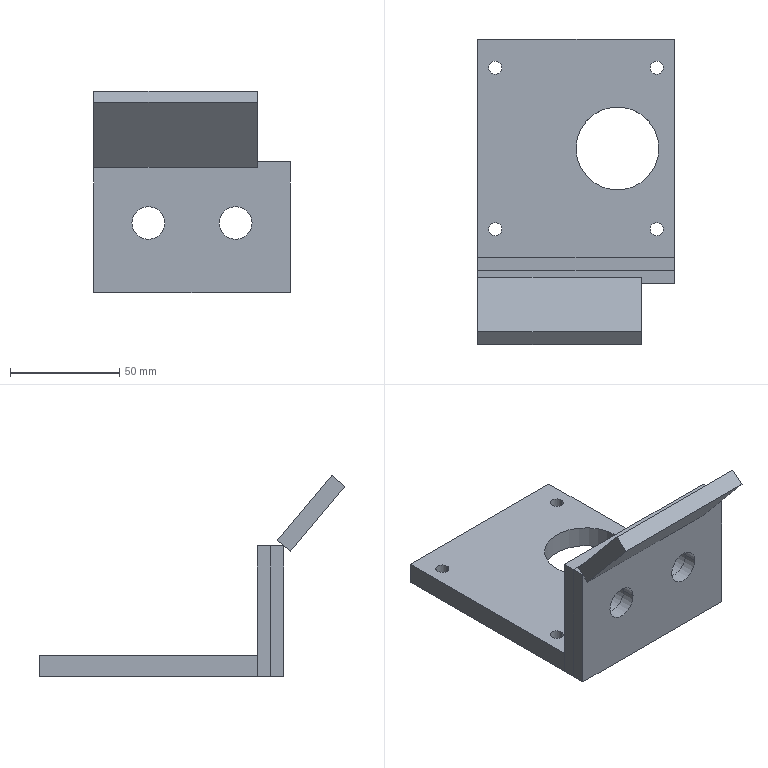Part | SolidWorks | features ICE 4, BossThin 1, Extrusion 1 | 4 solids | 42 faces | box 90 x 140.048 x 92.376 mm | volume 160839 mm3 | plane 24 | cylinder 18 | commonest cylinder face diameters 6 x8 15 x8 38 x2
STEP:
#1=CARTESIAN_POINT('',(-40.,-37.,10.));
#2=VERTEX_POINT('',#1);
#3=CARTESIAN_POINT('',(-34.,-37.,10.));
#4=VERTEX_POINT('',#3);
#5=CARTESIAN_POINT('',(-37.,-37.,10.));
#6=DIRECTION('',(0.,0.,1.));
#7=DIRECTION('',(-1.,0.,0.));
#8=AXIS2_PLACEMENT_3D('',#5,#6,#7);
#9=CIRCLE('',#8,3.);
#10=EDGE_CURVE('',#2,#4,#9,.T.);
#11=ORIENTED_EDGE('',*,*,#10,.T.);
#12=CARTESIAN_POINT('',(-34.,-37.,0.));
#13=VERTEX_POINT('',#12);
#14=CARTESIAN_POINT('',(-34.,-37.,10.));
#15=DIRECTION('',(0.,0.,-1.));
#16=VECTOR('',#15,1000.);
#17=LINE('',#14,#16);
#18=EDGE_CURVE('',#4,#13,#17,.T.);
#19=ORIENTED_EDGE('',*,*,#18,.T.);
#20=CARTESIAN_POINT('',(-40.,-37.,0.));
#21=VERTEX_POINT('',#20);
#22=CARTESIAN_POINT('',(-37.,-37.,0.));
#23=DIRECTION('',(0.,0.,1.));
#24=DIRECTION('',(-1.,0.,0.));
#25=AXIS2_PLACEMENT_3D('',#22,#23,#24);
#26=CIRCLE('',#25,3.);
#27=EDGE_CURVE('',#21,#13,#26,.T.);
#28=ORIENTED_EDGE('',*,*,#27,.F.);
#29=CARTESIAN_POINT('',(-40.,-37.,10.));
#30=DIRECTION('',(0.,0.,-1.));
#31=VECTOR('',#30,1000.);
#32=LINE('',#29,#31);
#33=EDGE_CURVE('',#2,#21,#32,.T.);
#34=ORIENTED_EDGE('',*,*,#33,.F.);
#35=EDGE_LOOP('',(#11,#19,#28,#34));
#36=FACE_OUTER_BOUND('',#35,.T.);
#37=CARTESIAN_POINT('',(-37.,-37.,10.));
#38=DIRECTION('',(0.,0.,-1.));
#39=DIRECTION('',(-1.,0.,0.));
#40=AXIS2_PLACEMENT_3D('',#37,#38,#39);
#41=CYLINDRICAL_SURFACE('',#40,3.);
#42=ADVANCED_FACE('',(#36),#41,.F.);
#43=CARTESIAN_POINT('',(34.,-37.,10.));
#44=VERTEX_POINT('',#43);
#45=CARTESIAN_POINT('',(40.,-37.,10.));
#46=VERTEX_POINT('',#45);
#47=CARTESIAN_POINT('',(37.,-37.,10.));
#48=DIRECTION('',(0.,0.,1.));
#49=DIRECTION('',(1.,0.,0.));
#50=AXIS2_PLACEMENT_3D('',#47,#48,#49);
#51=CIRCLE('',#50,3.);
#52=EDGE_CURVE('',#44,#46,#51,.T.);
#53=ORIENTED_EDGE('',*,*,#52,.T.);
#54=CARTESIAN_POINT('',(40.,-37.,0.));
#55=VERTEX_POINT('',#54);
#56=CARTESIAN_POINT('',(40.,-37.,10.));
#57=DIRECTION('',(0.,0.,-1.));
#58=VECTOR('',#57,1000.);
#59=LINE('',#56,#58);
#60=EDGE_CURVE('',#46,#55,#59,.T.);
#61=ORIENTED_EDGE('',*,*,#60,.T.);
#62=CARTESIAN_POINT('',(34.,-37.,0.));
#63=VERTEX_POINT('',#62);
#64=CARTESIAN_POINT('',(37.,-37.,0.));
#65=DIRECTION('',(0.,0.,1.));
#66=DIRECTION('',(1.,0.,0.));
#67=AXIS2_PLACEMENT_3D('',#64,#65,#66);
#68=CIRCLE('',#67,3.);
#69=EDGE_CURVE('',#63,#55,#68,.T.);
#70=ORIENTED_EDGE('',*,*,#69,.F.);
#71=CARTESIAN_POINT('',(34.,-37.,10.));
#72=DIRECTION('',(0.,0.,-1.));
#73=VECTOR('',#72,1000.);
#74=LINE('',#71,#73);
#75=EDGE_CURVE('',#44,#63,#74,.T.);
#76=ORIENTED_EDGE('',*,*,#75,.F.);
#77=EDGE_LOOP('',(#53,#61,#70,#76));
#78=FACE_OUTER_BOUND('',#77,.T.);
#79=CARTESIAN_POINT('',(37.,-37.,10.));
#80=DIRECTION('',(0.,0.,-1.));
#81=DIRECTION('',(-1.,0.,0.));
#82=AXIS2_PLACEMENT_3D('',#79,#80,#81);
#83=CYLINDRICAL_SURFACE('',#82,3.);
#84=ADVANCED_FACE('',(#78),#83,.F.);
#85=CARTESIAN_POINT('',(-40.,37.,10.));
#86=VERTEX_POINT('',#85);
#87=CARTESIAN_POINT('',(-34.,37.,10.));
#88=VERTEX_POINT('',#87);
#89=CARTESIAN_POINT('',(-37.,37.,10.));
#90=DIRECTION('',(0.,0.,1.));
#91=DIRECTION('',(1.,0.,0.));
#92=AXIS2_PLACEMENT_3D('',#89,#90,#91);
#93=CIRCLE('',#92,3.);
#94=EDGE_CURVE('',#86,#88,#93,.T.);
#95=ORIENTED_EDGE('',*,*,#94,.T.);
#96=CARTESIAN_POINT('',(-34.,37.,0.));
#97=VERTEX_POINT('',#96);
#98=CARTESIAN_POINT('',(-34.,37.,10.));
#99=DIRECTION('',(0.,0.,-1.));
#100=VECTOR('',#99,1000.);
#101=LINE('',#98,#100);
#102=EDGE_CURVE('',#88,#97,#101,.T.);
#103=ORIENTED_EDGE('',*,*,#102,.T.);
#104=CARTESIAN_POINT('',(-40.,37.,0.));
#105=VERTEX_POINT('',#104);
#106=CARTESIAN_POINT('',(-37.,37.,0.));
#107=DIRECTION('',(0.,0.,1.));
#108=DIRECTION('',(1.,0.,0.));
#109=AXIS2_PLACEMENT_3D('',#106,#107,#108);
#110=CIRCLE('',#109,3.);
#111=EDGE_CURVE('',#105,#97,#110,.T.);
#112=ORIENTED_EDGE('',*,*,#111,.F.);
#113=CARTESIAN_POINT('',(-40.,37.,10.));
#114=DIRECTION('',(0.,0.,-1.));
#115=VECTOR('',#114,1000.);
#116=LINE('',#113,#115);
#117=EDGE_CURVE('',#86,#105,#116,.T.);
#118=ORIENTED_EDGE('',*,*,#117,.F.);
#119=EDGE_LOOP('',(#95,#103,#112,#118));
#120=FACE_OUTER_BOUND('',#119,.T.);
#121=CARTESIAN_POINT('',(-37.,37.,10.));
#122=DIRECTION('',(0.,0.,-1.));
#123=DIRECTION('',(-1.,0.,0.));
#124=AXIS2_PLACEMENT_3D('',#121,#122,#123);
#125=CYLINDRICAL_SURFACE('',#124,3.);
#126=ADVANCED_FACE('',(#120),#125,.F.);
#127=CARTESIAN_POINT('',(34.,37.,10.));
#128=VERTEX_POINT('',#127);
#129=CARTESIAN_POINT('',(40.,37.,10.));
#130=VERTEX_POINT('',#129);
#131=CARTESIAN_POINT('',(37.,37.,10.));
#132=DIRECTION('',(0.,0.,1.));
#133=DIRECTION('',(-1.,0.,0.));
#134=AXIS2_PLACEMENT_3D('',#131,#132,#133);
#135=CIRCLE('',#134,3.);
#136=EDGE_CURVE('',#128,#130,#135,.T.);
#137=ORIENTED_EDGE('',*,*,#136,.T.);
#138=CARTESIAN_POINT('',(40.,37.,0.));
#139=VERTEX_POINT('',#138);
#140=CARTESIAN_POINT('',(40.,37.,10.));
#141=DIRECTION('',(0.,0.,-1.));
#142=VECTOR('',#141,1000.);
#143=LINE('',#140,#142);
#144=EDGE_CURVE('',#130,#139,#143,.T.);
#145=ORIENTED_EDGE('',*,*,#144,.T.);
#146=CARTESIAN_POINT('',(34.,37.,0.));
#147=VERTEX_POINT('',#146);
#148=CARTESIAN_POINT('',(37.,37.,0.));
#149=DIRECTION('',(0.,0.,1.));
#150=DIRECTION('',(-1.,0.,0.));
#151=AXIS2_PLACEMENT_3D('',#148,#149,#150);
#152=CIRCLE('',#151,3.);
#153=EDGE_CURVE('',#147,#139,#152,.T.);
#154=ORIENTED_EDGE('',*,*,#153,.F.);
#155=CARTESIAN_POINT('',(34.,37.,10.));
#156=DIRECTION('',(0.,0.,-1.));
#157=VECTOR('',#156,1000.);
#158=LINE('',#155,#157);
#159=EDGE_CURVE('',#128,#147,#158,.T.);
#160=ORIENTED_EDGE('',*,*,#159,.F.);
#161=EDGE_LOOP('',(#137,#145,#154,#160));
#162=FACE_OUTER_BOUND('',#161,.T.);
#163=CARTESIAN_POINT('',(37.,37.,10.));
#164=DIRECTION('',(0.,0.,-1.));
#165=DIRECTION('',(-1.,0.,0.));
#166=AXIS2_PLACEMENT_3D('',#163,#164,#165);
#167=CYLINDRICAL_SURFACE('',#166,3.);
#168=ADVANCED_FACE('',(#162),#167,.F.);
#169=CARTESIAN_POINT('',(0.,0.,10.));
#170=VERTEX_POINT('',#169);
#171=CARTESIAN_POINT('',(38.,0.,10.));
#172=VERTEX_POINT('',#171);
#173=CARTESIAN_POINT('',(19.,0.,10.));
#174=DIRECTION('',(0.,0.,1.));
#175=DIRECTION('',(1.,0.,0.));
#176=AXIS2_PLACEMENT_3D('',#173,#174,#175);
#177=CIRCLE('',#176,19.);
#178=EDGE_CURVE('',#170,#172,#177,.T.);
#179=ORIENTED_EDGE('',*,*,#178,.T.);
#180=CARTESIAN_POINT('',(38.,0.,0.));
#181=VERTEX_POINT('',#180);
#182=CARTESIAN_POINT('',(38.,0.,10.));
#183=DIRECTION('',(0.,0.,-1.));
#184=VECTOR('',#183,1000.);
#185=LINE('',#182,#184);
#186=EDGE_CURVE('',#172,#181,#185,.T.);
#187=ORIENTED_EDGE('',*,*,#186,.T.);
#188=CARTESIAN_POINT('',(0.,0.,0.));
#189=VERTEX_POINT('',#188);
#190=CARTESIAN_POINT('',(19.,0.,0.));
#191=DIRECTION('',(0.,0.,1.));
#192=DIRECTION('',(1.,0.,0.));
#193=AXIS2_PLACEMENT_3D('',#190,#191,#192);
#194=CIRCLE('',#193,19.);
#195=EDGE_CURVE('',#189,#181,#194,.T.);
#196=ORIENTED_EDGE('',*,*,#195,.F.);
#197=CARTESIAN_POINT('',(0.,0.,10.));
#198=DIRECTION('',(0.,0.,-1.));
#199=VECTOR('',#198,1000.);
#200=LINE('',#197,#199);
#201=EDGE_CURVE('',#170,#189,#200,.T.);
#202=ORIENTED_EDGE('',*,*,#201,.F.);
#203=EDGE_LOOP('',(#179,#187,#196,#202));
#204=FACE_OUTER_BOUND('',#203,.T.);
#205=CARTESIAN_POINT('',(19.,0.,10.));
#206=DIRECTION('',(0.,0.,-1.));
#207=DIRECTION('',(-1.,0.,0.));
#208=AXIS2_PLACEMENT_3D('',#205,#206,#207);
#209=CYLINDRICAL_SURFACE('',#208,19.);
#210=ADVANCED_FACE('',(#204),#209,.F.);
#211=CARTESIAN_POINT('',(45.,-50.,10.));
#212=VERTEX_POINT('',#211);
#213=CARTESIAN_POINT('',(45.,50.,10.));
#214=VERTEX_POINT('',#213);
#215=CARTESIAN_POINT('',(45.,-50.,10.));
#216=DIRECTION('',(0.,1.,0.));
#217=VECTOR('',#216,1000.);
#218=LINE('',#215,#217);
#219=EDGE_CURVE('',#212,#214,#218,.T.);
#220=ORIENTED_EDGE('',*,*,#219,.T.);
#221=CARTESIAN_POINT('',(-45.,50.,10.));
#222=VERTEX_POINT('',#221);
#223=CARTESIAN_POINT('',(-45.,50.,10.));
#224=DIRECTION('',(-1.,0.,0.));
#225=VECTOR('',#224,1000.);
#226=LINE('',#223,#225);
#227=EDGE_CURVE('',#214,#222,#226,.T.);
#228=ORIENTED_EDGE('',*,*,#227,.T.);
#229=CARTESIAN_POINT('',(-45.,-50.,10.));
#230=VERTEX_POINT('',#229);
#231=CARTESIAN_POINT('',(-45.,-50.,10.));
#232=DIRECTION('',(0.,-1.,0.));
#233=VECTOR('',#232,1000.);
#234=LINE('',#231,#233);
#235=EDGE_CURVE('',#222,#230,#234,.T.);
#236=ORIENTED_EDGE('',*,*,#235,.T.);
#237=CARTESIAN_POINT('',(-45.,-50.,10.));
#238=DIRECTION('',(1.,0.,0.));
#239=VECTOR('',#238,1000.);
#240=LINE('',#237,#239);
#241=EDGE_CURVE('',#230,#212,#240,.T.);
#242=ORIENTED_EDGE('',*,*,#241,.T.);
#243=EDGE_LOOP('',(#220,#228,#236,#242));
#244=FACE_OUTER_BOUND('',#243,.T.);
#245=ORIENTED_EDGE('',*,*,#178,.F.);
#246=CARTESIAN_POINT('',(19.,0.,10.));
#247=DIRECTION('',(0.,0.,1.));
#248=DIRECTION('',(1.,0.,0.));
#249=AXIS2_PLACEMENT_3D('',#246,#247,#248);
#250=CIRCLE('',#249,19.);
#251=EDGE_CURVE('',#172,#170,#250,.T.);
#252=ORIENTED_EDGE('',*,*,#251,.F.);
#253=EDGE_LOOP('',(#245,#252));
#254=FACE_BOUND('',#253,.T.);
#255=ORIENTED_EDGE('',*,*,#136,.F.);
#256=CARTESIAN_POINT('',(37.,37.,10.));
#257=DIRECTION('',(0.,0.,1.));
#258=DIRECTION('',(-1.,0.,0.));
#259=AXIS2_PLACEMENT_3D('',#256,#257,#258);
#260=CIRCLE('',#259,3.);
#261=EDGE_CURVE('',#130,#128,#260,.T.);
#262=ORIENTED_EDGE('',*,*,#261,.F.);
#263=EDGE_LOOP('',(#255,#262));
#264=FACE_BOUND('',#263,.T.);
#265=ORIENTED_EDGE('',*,*,#94,.F.);
#266=CARTESIAN_POINT('',(-37.,37.,10.));
#267=DIRECTION('',(0.,0.,1.));
#268=DIRECTION('',(1.,0.,0.));
#269=AXIS2_PLACEMENT_3D('',#266,#267,#268);
#270=CIRCLE('',#269,3.);
#271=EDGE_CURVE('',#88,#86,#270,.T.);
#272=ORIENTED_EDGE('',*,*,#271,.F.);
#273=EDGE_LOOP('',(#265,#272));
#274=FACE_BOUND('',#273,.T.);
#275=ORIENTED_EDGE('',*,*,#52,.F.);
#276=CARTESIAN_POINT('',(37.,-37.,10.));
#277=DIRECTION('',(0.,0.,1.));
#278=DIRECTION('',(1.,0.,0.));
#279=AXIS2_PLACEMENT_3D('',#276,#277,#278);
#280=CIRCLE('',#279,3.);
#281=EDGE_CURVE('',#46,#44,#280,.T.);
#282=ORIENTED_EDGE('',*,*,#281,.F.);
#283=EDGE_LOOP('',(#275,#282));
#284=FACE_BOUND('',#283,.T.);
#285=ORIENTED_EDGE('',*,*,#10,.F.);
#286=CARTESIAN_POINT('',(-37.,-37.,10.));
#287=DIRECTION('',(0.,0.,1.));
#288=DIRECTION('',(-1.,0.,0.));
#289=AXIS2_PLACEMENT_3D('',#286,#287,#288);
#290=CIRCLE('',#289,3.);
#291=EDGE_CURVE('',#4,#2,#290,.T.);
#292=ORIENTED_EDGE('',*,*,#291,.F.);
#293=EDGE_LOOP('',(#285,#292));
#294=FACE_BOUND('',#293,.T.);
#295=CARTESIAN_POINT('',(0.,0.,10.));
#296=DIRECTION('',(0.,0.,-1.));
#297=DIRECTION('',(-1.,0.,0.));
#298=AXIS2_PLACEMENT_3D('',#295,#296,#297);
#299=PLANE('',#298);
#300=ADVANCED_FACE('',(#244,#254,#264,#274,#284,#294),#299,.F.);
#301=ORIENTED_EDGE('',*,*,#69,.T.);
#302=CARTESIAN_POINT('',(37.,-37.,0.));
#303=DIRECTION('',(0.,0.,1.));
#304=DIRECTION('',(1.,0.,0.));
#305=AXIS2_PLACEMENT_3D('',#302,#303,#304);
#306=CIRCLE('',#305,3.);
#307=EDGE_CURVE('',#55,#63,#306,.T.);
#308=ORIENTED_EDGE('',*,*,#307,.T.);
#309=EDGE_LOOP('',(#301,#308));
#310=FACE_BOUND('',#309,.T.);
#311=ORIENTED_EDGE('',*,*,#153,.T.);
#312=CARTESIAN_POINT('',(37.,37.,0.));
#313=DIRECTION('',(0.,0.,1.));
#314=DIRECTION('',(-1.,0.,0.));
#315=AXIS2_PLACEMENT_3D('',#312,#313,#314);
#316=CIRCLE('',#315,3.);
#317=EDGE_CURVE('',#139,#147,#316,.T.);
#318=ORIENTED_EDGE('',*,*,#317,.T.);
#319=EDGE_LOOP('',(#311,#318));
#320=FACE_BOUND('',#319,.T.);
#321=CARTESIAN_POINT('',(45.,-50.,0.));
#322=VERTEX_POINT('',#321);
#323=CARTESIAN_POINT('',(45.,50.,0.));
#324=VERTEX_POINT('',#323);
#325=CARTESIAN_POINT('',(45.,-50.,0.));
#326=DIRECTION('',(0.,1.,0.));
#327=VECTOR('',#326,1000.);
#328=LINE('',#325,#327);
#329=EDGE_CURVE('',#322,#324,#328,.T.);
#330=ORIENTED_EDGE('',*,*,#329,.F.);
#331=CARTESIAN_POINT('',(-45.,-50.,0.));
#332=VERTEX_POINT('',#331);
#333=CARTESIAN_POINT('',(-45.,-50.,0.));
#334=DIRECTION('',(1.,0.,0.));
#335=VECTOR('',#334,1000.);
#336=LINE('',#333,#335);
#337=EDGE_CURVE('',#332,#322,#336,.T.);
#338=ORIENTED_EDGE('',*,*,#337,.F.);
#339=CARTESIAN_POINT('',(-45.,50.,0.));
#340=VERTEX_POINT('',#339);
#341=CARTESIAN_POINT('',(-45.,-50.,0.));
#342=DIRECTION('',(0.,-1.,0.));
#343=VECTOR('',#342,1000.);
#344=LINE('',#341,#343);
#345=EDGE_CURVE('',#340,#332,#344,.T.);
#346=ORIENTED_EDGE('',*,*,#345,.F.);
#347=CARTESIAN_POINT('',(-45.,50.,0.));
#348=DIRECTION('',(-1.,0.,0.));
#349=VECTOR('',#348,1000.);
#350=LINE('',#347,#349);
#351=EDGE_CURVE('',#324,#340,#350,.T.);
#352=ORIENTED_EDGE('',*,*,#351,.F.);
#353=EDGE_LOOP('',(#330,#338,#346,#352));
#354=FACE_OUTER_BOUND('',#353,.T.);
#355=ORIENTED_EDGE('',*,*,#195,.T.);
#356=CARTESIAN_POINT('',(19.,0.,0.));
#357=DIRECTION('',(0.,0.,1.));
#358=DIRECTION('',(1.,0.,0.));
#359=AXIS2_PLACEMENT_3D('',#356,#357,#358);
#360=CIRCLE('',#359,19.);
#361=EDGE_CURVE('',#181,#189,#360,.T.);
#362=ORIENTED_EDGE('',*,*,#361,.T.);
#363=EDGE_LOOP('',(#355,#362));
#364=FACE_BOUND('',#363,.T.);
#365=ORIENTED_EDGE('',*,*,#111,.T.);
#366=CARTESIAN_POINT('',(-37.,37.,0.));
#367=DIRECTION('',(0.,0.,1.));
#368=DIRECTION('',(1.,0.,0.));
#369=AXIS2_PLACEMENT_3D('',#366,#367,#368);
#370=CIRCLE('',#369,3.);
#371=EDGE_CURVE('',#97,#105,#370,.T.);
#372=ORIENTED_EDGE('',*,*,#371,.T.);
#373=EDGE_LOOP('',(#365,#372));
#374=FACE_BOUND('',#373,.T.);
#375=ORIENTED_EDGE('',*,*,#27,.T.);
#376=CARTESIAN_POINT('',(-37.,-37.,0.));
#377=DIRECTION('',(0.,0.,1.));
#378=DIRECTION('',(-1.,0.,0.));
#379=AXIS2_PLACEMENT_3D('',#376,#377,#378);
#380=CIRCLE('',#379,3.);
#381=EDGE_CURVE('',#13,#21,#380,.T.);
#382=ORIENTED_EDGE('',*,*,#381,.T.);
#383=EDGE_LOOP('',(#375,#382));
#384=FACE_BOUND('',#383,.T.);
#385=CARTESIAN_POINT('',(0.,0.,0.));
#386=DIRECTION('',(0.,0.,-1.));
#387=DIRECTION('',(-1.,0.,0.));
#388=AXIS2_PLACEMENT_3D('',#385,#386,#387);
#389=PLANE('',#388);
#390=ADVANCED_FACE('',(#310,#320,#354,#364,#374,#384),#389,.T.);
#391=ORIENTED_EDGE('',*,*,#329,.T.);
#392=CARTESIAN_POINT('',(45.,50.,10.));
#393=DIRECTION('',(0.,0.,-1.));
#394=VECTOR('',#393,1000.);
#395=LINE('',#392,#394);
#396=EDGE_CURVE('',#214,#324,#395,.T.);
#397=ORIENTED_EDGE('',*,*,#396,.F.);
#398=ORIENTED_EDGE('',*,*,#219,.F.);
#399=CARTESIAN_POINT('',(45.,-50.,10.));
#400=DIRECTION('',(0.,0.,-1.));
#401=VECTOR('',#400,1000.);
#402=LINE('',#399,#401);
#403=EDGE_CURVE('',#212,#322,#402,.T.);
#404=ORIENTED_EDGE('',*,*,#403,.T.);
#405=EDGE_LOOP('',(#391,#397,#398,#404));
#406=FACE_OUTER_BOUND('',#405,.T.);
#407=CARTESIAN_POINT('',(45.,-50.,10.));
#408=DIRECTION('',(-1.,0.,0.));
#409=DIRECTION('',(0.,0.,1.));
#410=AXIS2_PLACEMENT_3D('',#407,#408,#409);
#411=PLANE('',#410);
#412=ADVANCED_FACE('',(#406),#411,.F.);
#413=ORIENTED_EDGE('',*,*,#351,.T.);
#414=CARTESIAN_POINT('',(-45.,50.,10.));
#415=DIRECTION('',(0.,0.,-1.));
#416=VECTOR('',#415,1000.);
#417=LINE('',#414,#416);
#418=EDGE_CURVE('',#222,#340,#417,.T.);
#419=ORIENTED_EDGE('',*,*,#418,.F.);
#420=ORIENTED_EDGE('',*,*,#227,.F.);
#421=ORIENTED_EDGE('',*,*,#396,.T.);
#422=EDGE_LOOP('',(#413,#419,#420,#421));
#423=FACE_OUTER_BOUND('',#422,.T.);
#424=CARTESIAN_POINT('',(-45.,50.,10.));
#425=DIRECTION('',(0.,-1.,0.));
#426=DIRECTION('',(1.,0.,0.));
#427=AXIS2_PLACEMENT_3D('',#424,#425,#426);
#428=PLANE('',#427);
#429=ADVANCED_FACE('',(#423),#428,.F.);
#430=ORIENTED_EDGE('',*,*,#345,.T.);
#431=CARTESIAN_POINT('',(-45.,-50.,10.));
#432=DIRECTION('',(0.,0.,-1.));
#433=VECTOR('',#432,1000.);
#434=LINE('',#431,#433);
#435=EDGE_CURVE('',#230,#332,#434,.T.);
#436=ORIENTED_EDGE('',*,*,#435,.F.);
#437=ORIENTED_EDGE('',*,*,#235,.F.);
#438=ORIENTED_EDGE('',*,*,#418,.T.);
#439=EDGE_LOOP('',(#430,#436,#437,#438));
#440=FACE_OUTER_BOUND('',#439,.T.);
#441=CARTESIAN_POINT('',(-45.,-50.,10.));
#442=DIRECTION('',(1.,0.,0.));
#443=DIRECTION('',(0.,1.,0.));
#444=AXIS2_PLACEMENT_3D('',#441,#442,#443);
#445=PLANE('',#444);
#446=ADVANCED_FACE('',(#440),#445,.F.);
#447=ORIENTED_EDGE('',*,*,#337,.T.);
#448=ORIENTED_EDGE('',*,*,#403,.F.);
#449=ORIENTED_EDGE('',*,*,#241,.F.);
#450=ORIENTED_EDGE('',*,*,#435,.T.);
#451=EDGE_LOOP('',(#447,#448,#449,#450));
#452=FACE_OUTER_BOUND('',#451,.T.);
#453=CARTESIAN_POINT('',(-45.,-50.,10.));
#454=DIRECTION('',(0.,1.,0.));
#455=DIRECTION('',(-1.,0.,0.));
#456=AXIS2_PLACEMENT_3D('',#453,#454,#455);
#457=PLANE('',#456);
#458=ADVANCED_FACE('',(#452),#457,.F.);
#459=ORIENTED_EDGE('',*,*,#186,.F.);
#460=ORIENTED_EDGE('',*,*,#251,.T.);
#461=ORIENTED_EDGE('',*,*,#201,.T.);
#462=ORIENTED_EDGE('',*,*,#361,.F.);
#463=EDGE_LOOP('',(#459,#460,#461,#462));
#464=FACE_OUTER_BOUND('',#463,.T.);
#465=CARTESIAN_POINT('',(19.,0.,10.));
#466=DIRECTION('',(0.,0.,-1.));
#467=DIRECTION('',(-1.,0.,0.));
#468=AXIS2_PLACEMENT_3D('',#465,#466,#467);
#469=CYLINDRICAL_SURFACE('',#468,19.);
#470=ADVANCED_FACE('',(#464),#469,.F.);
#471=ORIENTED_EDGE('',*,*,#144,.F.);
#472=ORIENTED_EDGE('',*,*,#261,.T.);
#473=ORIENTED_EDGE('',*,*,#159,.T.);
#474=ORIENTED_EDGE('',*,*,#317,.F.);
#475=EDGE_LOOP('',(#471,#472,#473,#474));
#476=FACE_OUTER_BOUND('',#475,.T.);
#477=CARTESIAN_POINT('',(37.,37.,10.));
#478=DIRECTION('',(0.,0.,-1.));
#479=DIRECTION('',(-1.,0.,0.));
#480=AXIS2_PLACEMENT_3D('',#477,#478,#479);
#481=CYLINDRICAL_SURFACE('',#480,3.);
#482=ADVANCED_FACE('',(#476),#481,.F.);
#483=ORIENTED_EDGE('',*,*,#102,.F.);
#484=ORIENTED_EDGE('',*,*,#271,.T.);
#485=ORIENTED_EDGE('',*,*,#117,.T.);
#486=ORIENTED_EDGE('',*,*,#371,.F.);
#487=EDGE_LOOP('',(#483,#484,#485,#486));
#488=FACE_OUTER_BOUND('',#487,.T.);
#489=CARTESIAN_POINT('',(-37.,37.,10.));
#490=DIRECTION('',(0.,0.,-1.));
#491=DIRECTION('',(-1.,0.,0.));
#492=AXIS2_PLACEMENT_3D('',#489,#490,#491);
#493=CYLINDRICAL_SURFACE('',#492,3.);
#494=ADVANCED_FACE('',(#488),#493,.F.);
#495=ORIENTED_EDGE('',*,*,#60,.F.);
#496=ORIENTED_EDGE('',*,*,#281,.T.);
#497=ORIENTED_EDGE('',*,*,#75,.T.);
#498=ORIENTED_EDGE('',*,*,#307,.F.);
#499=EDGE_LOOP('',(#495,#496,#497,#498));
#500=FACE_OUTER_BOUND('',#499,.T.);
#501=CARTESIAN_POINT('',(37.,-37.,10.));
#502=DIRECTION('',(0.,0.,-1.));
#503=DIRECTION('',(-1.,0.,0.));
#504=AXIS2_PLACEMENT_3D('',#501,#502,#503);
#505=CYLINDRICAL_SURFACE('',#504,3.);
#506=ADVANCED_FACE('',(#500),#505,.F.);
#507=ORIENTED_EDGE('',*,*,#18,.F.);
#508=ORIENTED_EDGE('',*,*,#291,.T.);
#509=ORIENTED_EDGE('',*,*,#33,.T.);
#510=ORIENTED_EDGE('',*,*,#381,.F.);
#511=EDGE_LOOP('',(#507,#508,#509,#510));
#512=FACE_OUTER_BOUND('',#511,.T.);
#513=CARTESIAN_POINT('',(-37.,-37.,10.));
#514=DIRECTION('',(0.,0.,-1.));
#515=DIRECTION('',(-1.,0.,0.));
#516=AXIS2_PLACEMENT_3D('',#513,#514,#515);
#517=CYLINDRICAL_SURFACE('',#516,3.);
#518=ADVANCED_FACE('',(#512),#517,.F.);
#519=CLOSED_SHELL('',(#42,#84,#126,#168,#210,#300,#390,#412,#429,#446,#458,#470,#482,#494,#506,#518));
#520=MANIFOLD_SOLID_BREP('',#519);
#521=CARTESIAN_POINT('',(27.5,-50.,32.));
#522=VERTEX_POINT('',#521);
#523=CARTESIAN_POINT('',(12.5,-50.,32.));
#524=VERTEX_POINT('',#523);
#525=CARTESIAN_POINT('',(20.,-50.,32.));
#526=DIRECTION('',(0.,1.,0.));
#527=DIRECTION('',(-1.,0.,0.));
#528=AXIS2_PLACEMENT_3D('',#525,#526,#527);
#529=CIRCLE('',#528,7.5);
#530=EDGE_CURVE('',#522,#524,#529,.T.);
#531=ORIENTED_EDGE('',*,*,#530,.T.);
#532=CARTESIAN_POINT('',(12.5,-56.,32.));
#533=VERTEX_POINT('',#532);
#534=CARTESIAN_POINT('',(12.5,50.,32.));
#535=DIRECTION('',(0.,-1.,0.));
#536=VECTOR('',#535,1000.);
#537=LINE('',#534,#536);
#538=EDGE_CURVE('',#524,#533,#537,.T.);
#539=ORIENTED_EDGE('',*,*,#538,.T.);
#540=CARTESIAN_POINT('',(27.5,-56.,32.));
#541=VERTEX_POINT('',#540);
#542=CARTESIAN_POINT('',(20.,-56.,32.));
#543=DIRECTION('',(0.,1.,0.));
#544=DIRECTION('',(-1.,0.,0.));
#545=AXIS2_PLACEMENT_3D('',#542,#543,#544);
#546=CIRCLE('',#545,7.5);
#547=EDGE_CURVE('',#541,#533,#546,.T.);
#548=ORIENTED_EDGE('',*,*,#547,.F.);
#549=CARTESIAN_POINT('',(27.5,50.,32.));
#550=DIRECTION('',(0.,-1.,0.));
#551=VECTOR('',#550,1000.);
#552=LINE('',#549,#551);
#553=EDGE_CURVE('',#522,#541,#552,.T.);
#554=ORIENTED_EDGE('',*,*,#553,.F.);
#555=EDGE_LOOP('',(#531,#539,#548,#554));
#556=FACE_OUTER_BOUND('',#555,.T.);
#557=CARTESIAN_POINT('',(20.,50.,32.));
#558=DIRECTION('',(0.,-1.,0.));
#559=DIRECTION('',(1.,0.,0.));
#560=AXIS2_PLACEMENT_3D('',#557,#558,#559);
#561=CYLINDRICAL_SURFACE('',#560,7.5);
#562=ADVANCED_FACE('',(#556),#561,.F.);
#563=CARTESIAN_POINT('',(-12.5,-50.,32.));
#564=VERTEX_POINT('',#563);
#565=CARTESIAN_POINT('',(-27.5,-50.,32.));
#566=VERTEX_POINT('',#565);
#567=CARTESIAN_POINT('',(-20.,-50.,32.));
#568=DIRECTION('',(0.,1.,0.));
#569=DIRECTION('',(-1.,0.,0.));
#570=AXIS2_PLACEMENT_3D('',#567,#568,#569);
#571=CIRCLE('',#570,7.5);
#572=EDGE_CURVE('',#564,#566,#571,.T.);
#573=ORIENTED_EDGE('',*,*,#572,.T.);
#574=CARTESIAN_POINT('',(-27.5,-56.,32.));
#575=VERTEX_POINT('',#574);
#576=CARTESIAN_POINT('',(-27.5,50.,32.));
#577=DIRECTION('',(0.,-1.,0.));
#578=VECTOR('',#577,1000.);
#579=LINE('',#576,#578);
#580=EDGE_CURVE('',#566,#575,#579,.T.);
#581=ORIENTED_EDGE('',*,*,#580,.T.);
#582=CARTESIAN_POINT('',(-12.5,-56.,32.));
#583=VERTEX_POINT('',#582);
#584=CARTESIAN_POINT('',(-20.,-56.,32.));
#585=DIRECTION('',(0.,1.,0.));
#586=DIRECTION('',(-1.,0.,0.));
#587=AXIS2_PLACEMENT_3D('',#584,#585,#586);
#588=CIRCLE('',#587,7.5);
#589=EDGE_CURVE('',#583,#575,#588,.T.);
#590=ORIENTED_EDGE('',*,*,#589,.F.);
#591=CARTESIAN_POINT('',(-12.5,50.,32.));
#592=DIRECTION('',(0.,-1.,0.));
#593=VECTOR('',#592,1000.);
#594=LINE('',#591,#593);
#595=EDGE_CURVE('',#564,#583,#594,.T.);
#596=ORIENTED_EDGE('',*,*,#595,.F.);
#597=EDGE_LOOP('',(#573,#581,#590,#596));
#598=FACE_OUTER_BOUND('',#597,.T.);
#599=CARTESIAN_POINT('',(-20.,50.,32.));
#600=DIRECTION('',(0.,-1.,0.));
#601=DIRECTION('',(1.,0.,0.));
#602=AXIS2_PLACEMENT_3D('',#599,#600,#601);
#603=CYLINDRICAL_SURFACE('',#602,7.5);
#604=ADVANCED_FACE('',(#598),#603,.F.);
#605=CARTESIAN_POINT('',(-45.,-50.,0.));
#606=VERTEX_POINT('',#605);
#607=CARTESIAN_POINT('',(-45.,-50.,60.));
#608=VERTEX_POINT('',#607);
#609=CARTESIAN_POINT('',(-45.,-50.,0.));
#610=DIRECTION('',(0.,0.,1.));
#611=VECTOR('',#610,1000.);
#612=LINE('',#609,#611);
#613=EDGE_CURVE('',#606,#608,#612,.T.);
#614=ORIENTED_EDGE('',*,*,#613,.F.);
#615=CARTESIAN_POINT('',(-45.,-56.,0.));
#616=VERTEX_POINT('',#615);
#617=CARTESIAN_POINT('',(-45.,-56.,0.));
#618=DIRECTION('',(0.,1.,0.));
#619=VECTOR('',#618,1000.);
#620=LINE('',#617,#619);
#621=EDGE_CURVE('',#616,#606,#620,.T.);
#622=ORIENTED_EDGE('',*,*,#621,.F.);
#623=CARTESIAN_POINT('',(-45.,-56.,60.));
#624=VERTEX_POINT('',#623);
#625=CARTESIAN_POINT('',(-45.,-56.,0.));
#626=DIRECTION('',(0.,0.,1.));
#627=VECTOR('',#626,1000.);
#628=LINE('',#625,#627);
#629=EDGE_CURVE('',#616,#624,#628,.T.);
#630=ORIENTED_EDGE('',*,*,#629,.T.);
#631=CARTESIAN_POINT('',(-45.,-56.,60.));
#632=DIRECTION('',(0.,1.,0.));
#633=VECTOR('',#632,1000.);
#634=LINE('',#631,#633);
#635=EDGE_CURVE('',#624,#608,#634,.T.);
#636=ORIENTED_EDGE('',*,*,#635,.T.);
#637=EDGE_LOOP('',(#614,#622,#630,#636));
#638=FACE_OUTER_BOUND('',#637,.T.);
#639=CARTESIAN_POINT('',(-45.,-56.,0.));
#640=DIRECTION('',(-1.,0.,0.));
#641=DIRECTION('',(0.,-1.,0.));
#642=AXIS2_PLACEMENT_3D('',#639,#640,#641);
#643=PLANE('',#642);
#644=ADVANCED_FACE('',(#638),#643,.T.);
#645=CARTESIAN_POINT('',(45.,-50.,0.));
#646=VERTEX_POINT('',#645);
#647=CARTESIAN_POINT('',(-45.,-50.,0.));
#648=DIRECTION('',(-1.,0.,0.));
#649=VECTOR('',#648,1000.);
#650=LINE('',#647,#649);
#651=EDGE_CURVE('',#646,#606,#650,.T.);
#652=ORIENTED_EDGE('',*,*,#651,.F.);
#653=CARTESIAN_POINT('',(45.,-56.,0.));
#654=VERTEX_POINT('',#653);
#655=CARTESIAN_POINT('',(45.,-56.,0.));
#656=DIRECTION('',(0.,1.,0.));
#657=VECTOR('',#656,1000.);
#658=LINE('',#655,#657);
#659=EDGE_CURVE('',#654,#646,#658,.T.);
#660=ORIENTED_EDGE('',*,*,#659,.F.);
#661=CARTESIAN_POINT('',(-45.,-56.,0.));
#662=DIRECTION('',(-1.,0.,0.));
#663=VECTOR('',#662,1000.);
#664=LINE('',#661,#663);
#665=EDGE_CURVE('',#654,#616,#664,.T.);
#666=ORIENTED_EDGE('',*,*,#665,.T.);
#667=ORIENTED_EDGE('',*,*,#621,.T.);
#668=EDGE_LOOP('',(#652,#660,#666,#667));
#669=FACE_OUTER_BOUND('',#668,.T.);
#670=CARTESIAN_POINT('',(-45.,-56.,0.));
#671=DIRECTION('',(0.,0.,-1.));
#672=DIRECTION('',(-1.,0.,0.));
#673=AXIS2_PLACEMENT_3D('',#670,#671,#672);
#674=PLANE('',#673);
#675=ADVANCED_FACE('',(#669),#674,.T.);
#676=CARTESIAN_POINT('',(45.,-50.,60.));
#677=VERTEX_POINT('',#676);
#678=CARTESIAN_POINT('',(45.,-50.,0.));
#679=DIRECTION('',(0.,0.,-1.));
#680=VECTOR('',#679,1000.);
#681=LINE('',#678,#680);
#682=EDGE_CURVE('',#677,#646,#681,.T.);
#683=ORIENTED_EDGE('',*,*,#682,.F.);
#684=CARTESIAN_POINT('',(45.,-56.,60.));
#685=VERTEX_POINT('',#684);
#686=CARTESIAN_POINT('',(45.,-56.,60.));
#687=DIRECTION('',(0.,1.,0.));
#688=VECTOR('',#687,1000.);
#689=LINE('',#686,#688);
#690=EDGE_CURVE('',#685,#677,#689,.T.);
#691=ORIENTED_EDGE('',*,*,#690,.F.);
#692=CARTESIAN_POINT('',(45.,-56.,0.));
#693=DIRECTION('',(0.,0.,-1.));
#694=VECTOR('',#693,1000.);
#695=LINE('',#692,#694);
#696=EDGE_CURVE('',#685,#654,#695,.T.);
#697=ORIENTED_EDGE('',*,*,#696,.T.);
#698=ORIENTED_EDGE('',*,*,#659,.T.);
#699=EDGE_LOOP('',(#683,#691,#697,#698));
#700=FACE_OUTER_BOUND('',#699,.T.);
#701=CARTESIAN_POINT('',(45.,-56.,0.));
#702=DIRECTION('',(1.,0.,0.));
#703=DIRECTION('',(0.,0.,-1.));
#704=AXIS2_PLACEMENT_3D('',#701,#702,#703);
#705=PLANE('',#704);
#706=ADVANCED_FACE('',(#700),#705,.T.);
#707=CARTESIAN_POINT('',(-45.,-50.,60.));
#708=DIRECTION('',(1.,0.,0.));
#709=VECTOR('',#708,1000.);
#710=LINE('',#707,#709);
#711=EDGE_CURVE('',#608,#677,#710,.T.);
#712=ORIENTED_EDGE('',*,*,#711,.F.);
#713=ORIENTED_EDGE('',*,*,#635,.F.);
#714=CARTESIAN_POINT('',(-45.,-56.,60.));
#715=DIRECTION('',(1.,0.,0.));
#716=VECTOR('',#715,1000.);
#717=LINE('',#714,#716);
#718=EDGE_CURVE('',#624,#685,#717,.T.);
#719=ORIENTED_EDGE('',*,*,#718,.T.);
#720=ORIENTED_EDGE('',*,*,#690,.T.);
#721=EDGE_LOOP('',(#712,#713,#719,#720));
#722=FACE_OUTER_BOUND('',#721,.T.);
#723=CARTESIAN_POINT('',(-45.,-56.,60.));
#724=DIRECTION('',(0.,0.,1.));
#725=DIRECTION('',(1.,0.,0.));
#726=AXIS2_PLACEMENT_3D('',#723,#724,#725);
#727=PLANE('',#726);
#728=ADVANCED_FACE('',(#722),#727,.T.);
#729=ORIENTED_EDGE('',*,*,#547,.T.);
#730=CARTESIAN_POINT('',(20.,-56.,32.));
#731=DIRECTION('',(0.,1.,0.));
#732=DIRECTION('',(-1.,0.,0.));
#733=AXIS2_PLACEMENT_3D('',#730,#731,#732);
#734=CIRCLE('',#733,7.5);
#735=EDGE_CURVE('',#533,#541,#734,.T.);
#736=ORIENTED_EDGE('',*,*,#735,.T.);
#737=EDGE_LOOP('',(#729,#736));
#738=FACE_BOUND('',#737,.T.);
#739=ORIENTED_EDGE('',*,*,#589,.T.);
#740=CARTESIAN_POINT('',(-20.,-56.,32.));
#741=DIRECTION('',(0.,1.,0.));
#742=DIRECTION('',(-1.,0.,0.));
#743=AXIS2_PLACEMENT_3D('',#740,#741,#742);
#744=CIRCLE('',#743,7.5);
#745=EDGE_CURVE('',#575,#583,#744,.T.);
#746=ORIENTED_EDGE('',*,*,#745,.T.);
#747=EDGE_LOOP('',(#739,#746));
#748=FACE_BOUND('',#747,.T.);
#749=ORIENTED_EDGE('',*,*,#629,.F.);
#750=ORIENTED_EDGE('',*,*,#665,.F.);
#751=ORIENTED_EDGE('',*,*,#696,.F.);
#752=ORIENTED_EDGE('',*,*,#718,.F.);
#753=EDGE_LOOP('',(#749,#750,#751,#752));
#754=FACE_OUTER_BOUND('',#753,.T.);
#755=CARTESIAN_POINT('',(0.,-56.,0.));
#756=DIRECTION('',(0.,1.,0.));
#757=DIRECTION('',(-1.,0.,0.));
#758=AXIS2_PLACEMENT_3D('',#755,#756,#757);
#759=PLANE('',#758);
#760=ADVANCED_FACE('',(#738,#748,#754),#759,.F.);
#761=ORIENTED_EDGE('',*,*,#530,.F.);
#762=CARTESIAN_POINT('',(20.,-50.,32.));
#763=DIRECTION('',(0.,1.,0.));
#764=DIRECTION('',(-1.,0.,0.));
#765=AXIS2_PLACEMENT_3D('',#762,#763,#764);
#766=CIRCLE('',#765,7.5);
#767=EDGE_CURVE('',#524,#522,#766,.T.);
#768=ORIENTED_EDGE('',*,*,#767,.F.);
#769=EDGE_LOOP('',(#761,#768));
#770=FACE_BOUND('',#769,.T.);
#771=ORIENTED_EDGE('',*,*,#572,.F.);
#772=CARTESIAN_POINT('',(-20.,-50.,32.));
#773=DIRECTION('',(0.,1.,0.));
#774=DIRECTION('',(-1.,0.,0.));
#775=AXIS2_PLACEMENT_3D('',#772,#773,#774);
#776=CIRCLE('',#775,7.5);
#777=EDGE_CURVE('',#566,#564,#776,.T.);
#778=ORIENTED_EDGE('',*,*,#777,.F.);
#779=EDGE_LOOP('',(#771,#778));
#780=FACE_BOUND('',#779,.T.);
#781=ORIENTED_EDGE('',*,*,#613,.T.);
#782=ORIENTED_EDGE('',*,*,#711,.T.);
#783=ORIENTED_EDGE('',*,*,#682,.T.);
#784=ORIENTED_EDGE('',*,*,#651,.T.);
#785=EDGE_LOOP('',(#781,#782,#783,#784));
#786=FACE_OUTER_BOUND('',#785,.T.);
#787=CARTESIAN_POINT('',(0.,-50.,0.));
#788=DIRECTION('',(0.,1.,0.));
#789=DIRECTION('',(-1.,0.,0.));
#790=AXIS2_PLACEMENT_3D('',#787,#788,#789);
#791=PLANE('',#790);
#792=ADVANCED_FACE('',(#770,#780,#786),#791,.T.);
#793=ORIENTED_EDGE('',*,*,#580,.F.);
#794=ORIENTED_EDGE('',*,*,#777,.T.);
#795=ORIENTED_EDGE('',*,*,#595,.T.);
#796=ORIENTED_EDGE('',*,*,#745,.F.);
#797=EDGE_LOOP('',(#793,#794,#795,#796));
#798=FACE_OUTER_BOUND('',#797,.T.);
#799=CARTESIAN_POINT('',(-20.,50.,32.));
#800=DIRECTION('',(0.,-1.,0.));
#801=DIRECTION('',(1.,0.,0.));
#802=AXIS2_PLACEMENT_3D('',#799,#800,#801);
#803=CYLINDRICAL_SURFACE('',#802,7.5);
#804=ADVANCED_FACE('',(#798),#803,.F.);
#805=ORIENTED_EDGE('',*,*,#538,.F.);
#806=ORIENTED_EDGE('',*,*,#767,.T.);
#807=ORIENTED_EDGE('',*,*,#553,.T.);
#808=ORIENTED_EDGE('',*,*,#735,.F.);
#809=EDGE_LOOP('',(#805,#806,#807,#808));
#810=FACE_OUTER_BOUND('',#809,.T.);
#811=CARTESIAN_POINT('',(20.,50.,32.));
#812=DIRECTION('',(0.,-1.,0.));
#813=DIRECTION('',(1.,0.,0.));
#814=AXIS2_PLACEMENT_3D('',#811,#812,#813);
#815=CYLINDRICAL_SURFACE('',#814,7.5);
#816=ADVANCED_FACE('',(#810),#815,.F.);
#817=CLOSED_SHELL('',(#562,#604,#644,#675,#706,#728,#760,#792,#804,#816));
#818=MANIFOLD_SOLID_BREP('',#817);
#819=CARTESIAN_POINT('',(12.5,-56.,32.));
#820=VERTEX_POINT('',#819);
#821=CARTESIAN_POINT('',(27.5,-56.,32.));
#822=VERTEX_POINT('',#821);
#823=CARTESIAN_POINT('',(20.,-56.,32.));
#824=DIRECTION('',(0.,-1.,0.));
#825=DIRECTION('',(1.,0.,0.));
#826=AXIS2_PLACEMENT_3D('',#823,#824,#825);
#827=CIRCLE('',#826,7.5);
#828=EDGE_CURVE('',#820,#822,#827,.T.);
#829=ORIENTED_EDGE('',*,*,#828,.F.);
#830=CARTESIAN_POINT('',(12.5,-62.,32.));
#831=VERTEX_POINT('',#830);
#832=CARTESIAN_POINT('',(12.5,50.,32.));
#833=DIRECTION('',(0.,-1.,0.));
#834=VECTOR('',#833,1000.);
#835=LINE('',#832,#834);
#836=EDGE_CURVE('',#820,#831,#835,.T.);
#837=ORIENTED_EDGE('',*,*,#836,.T.);
#838=CARTESIAN_POINT('',(27.5,-62.,32.));
#839=VERTEX_POINT('',#838);
#840=CARTESIAN_POINT('',(20.,-62.,32.));
#841=DIRECTION('',(0.,-1.,0.));
#842=DIRECTION('',(1.,0.,0.));
#843=AXIS2_PLACEMENT_3D('',#840,#841,#842);
#844=CIRCLE('',#843,7.5);
#845=EDGE_CURVE('',#831,#839,#844,.T.);
#846=ORIENTED_EDGE('',*,*,#845,.T.);
#847=CARTESIAN_POINT('',(27.5,50.,32.));
#848=DIRECTION('',(0.,-1.,0.));
#849=VECTOR('',#848,1000.);
#850=LINE('',#847,#849);
#851=EDGE_CURVE('',#822,#839,#850,.T.);
#852=ORIENTED_EDGE('',*,*,#851,.F.);
#853=EDGE_LOOP('',(#829,#837,#846,#852));
#854=FACE_OUTER_BOUND('',#853,.T.);
#855=CARTESIAN_POINT('',(20.,50.,32.));
#856=DIRECTION('',(0.,-1.,0.));
#857=DIRECTION('',(1.,0.,0.));
#858=AXIS2_PLACEMENT_3D('',#855,#856,#857);
#859=CYLINDRICAL_SURFACE('',#858,7.5);
#860=ADVANCED_FACE('',(#854),#859,.F.);
#861=CARTESIAN_POINT('',(-27.5,-56.,32.));
#862=VERTEX_POINT('',#861);
#863=CARTESIAN_POINT('',(-12.5,-56.,32.));
#864=VERTEX_POINT('',#863);
#865=CARTESIAN_POINT('',(-20.,-56.,32.));
#866=DIRECTION('',(0.,-1.,0.));
#867=DIRECTION('',(1.,0.,0.));
#868=AXIS2_PLACEMENT_3D('',#865,#866,#867);
#869=CIRCLE('',#868,7.5);
#870=EDGE_CURVE('',#862,#864,#869,.T.);
#871=ORIENTED_EDGE('',*,*,#870,.F.);
#872=CARTESIAN_POINT('',(-27.5,-62.,32.));
#873=VERTEX_POINT('',#872);
#874=CARTESIAN_POINT('',(-27.5,50.,32.));
#875=DIRECTION('',(0.,-1.,0.));
#876=VECTOR('',#875,1000.);
#877=LINE('',#874,#876);
#878=EDGE_CURVE('',#862,#873,#877,.T.);
#879=ORIENTED_EDGE('',*,*,#878,.T.);
#880=CARTESIAN_POINT('',(-12.5,-62.,32.));
#881=VERTEX_POINT('',#880);
#882=CARTESIAN_POINT('',(-20.,-62.,32.));
#883=DIRECTION('',(0.,-1.,0.));
#884=DIRECTION('',(-1.,0.,0.));
#885=AXIS2_PLACEMENT_3D('',#882,#883,#884);
#886=CIRCLE('',#885,7.5);
#887=EDGE_CURVE('',#873,#881,#886,.T.);
#888=ORIENTED_EDGE('',*,*,#887,.T.);
#889=CARTESIAN_POINT('',(-12.5,50.,32.));
#890=DIRECTION('',(0.,-1.,0.));
#891=VECTOR('',#890,1000.);
#892=LINE('',#889,#891);
#893=EDGE_CURVE('',#864,#881,#892,.T.);
#894=ORIENTED_EDGE('',*,*,#893,.F.);
#895=EDGE_LOOP('',(#871,#879,#888,#894));
#896=FACE_OUTER_BOUND('',#895,.T.);
#897=CARTESIAN_POINT('',(-20.,50.,32.));
#898=DIRECTION('',(0.,-1.,0.));
#899=DIRECTION('',(1.,0.,0.));
#900=AXIS2_PLACEMENT_3D('',#897,#898,#899);
#901=CYLINDRICAL_SURFACE('',#900,7.5);
#902=ADVANCED_FACE('',(#896),#901,.F.);
#903=CARTESIAN_POINT('',(45.,-56.,0.));
#904=VERTEX_POINT('',#903);
#905=CARTESIAN_POINT('',(45.,-56.,60.));
#906=VERTEX_POINT('',#905);
#907=CARTESIAN_POINT('',(45.,-56.,0.));
#908=DIRECTION('',(0.,0.,1.));
#909=VECTOR('',#908,1000.);
#910=LINE('',#907,#909);
#911=EDGE_CURVE('',#904,#906,#910,.T.);
#912=ORIENTED_EDGE('',*,*,#911,.T.);
#913=CARTESIAN_POINT('',(45.,-62.,60.));
#914=VERTEX_POINT('',#913);
#915=CARTESIAN_POINT('',(45.,-62.,60.));
#916=DIRECTION('',(0.,1.,0.));
#917=VECTOR('',#916,1000.);
#918=LINE('',#915,#917);
#919=EDGE_CURVE('',#914,#906,#918,.T.);
#920=ORIENTED_EDGE('',*,*,#919,.F.);
#921=CARTESIAN_POINT('',(45.,-62.,0.));
#922=VERTEX_POINT('',#921);
#923=CARTESIAN_POINT('',(45.,-62.,0.));
#924=DIRECTION('',(0.,0.,1.));
#925=VECTOR('',#924,1000.);
#926=LINE('',#923,#925);
#927=EDGE_CURVE('',#922,#914,#926,.T.);
#928=ORIENTED_EDGE('',*,*,#927,.F.);
#929=CARTESIAN_POINT('',(45.,-62.,0.));
#930=DIRECTION('',(0.,1.,0.));
#931=VECTOR('',#930,1000.);
#932=LINE('',#929,#931);
#933=EDGE_CURVE('',#922,#904,#932,.T.);
#934=ORIENTED_EDGE('',*,*,#933,.T.);
#935=EDGE_LOOP('',(#912,#920,#928,#934));
#936=FACE_OUTER_BOUND('',#935,.T.);
#937=CARTESIAN_POINT('',(45.,-62.,0.));
#938=DIRECTION('',(-1.,0.,0.));
#939=DIRECTION('',(0.,0.,1.));
#940=AXIS2_PLACEMENT_3D('',#937,#938,#939);
#941=PLANE('',#940);
#942=ADVANCED_FACE('',(#936),#941,.F.);
#943=CARTESIAN_POINT('',(-45.,-56.,60.));
#944=VERTEX_POINT('',#943);
#945=CARTESIAN_POINT('',(45.,-56.,60.));
#946=DIRECTION('',(-1.,0.,0.));
#947=VECTOR('',#946,1000.);
#948=LINE('',#945,#947);
#949=EDGE_CURVE('',#906,#944,#948,.T.);
#950=ORIENTED_EDGE('',*,*,#949,.T.);
#951=CARTESIAN_POINT('',(-45.,-62.,60.));
#952=VERTEX_POINT('',#951);
#953=CARTESIAN_POINT('',(-45.,-62.,60.));
#954=DIRECTION('',(0.,1.,0.));
#955=VECTOR('',#954,1000.);
#956=LINE('',#953,#955);
#957=EDGE_CURVE('',#952,#944,#956,.T.);
#958=ORIENTED_EDGE('',*,*,#957,.F.);
#959=CARTESIAN_POINT('',(45.,-62.,60.));
#960=DIRECTION('',(-1.,0.,0.));
#961=VECTOR('',#960,1000.);
#962=LINE('',#959,#961);
#963=EDGE_CURVE('',#914,#952,#962,.T.);
#964=ORIENTED_EDGE('',*,*,#963,.F.);
#965=ORIENTED_EDGE('',*,*,#919,.T.);
#966=EDGE_LOOP('',(#950,#958,#964,#965));
#967=FACE_OUTER_BOUND('',#966,.T.);
#968=CARTESIAN_POINT('',(45.,-62.,60.));
#969=DIRECTION('',(0.,0.,-1.));
#970=DIRECTION('',(0.,1.,0.));
#971=AXIS2_PLACEMENT_3D('',#968,#969,#970);
#972=PLANE('',#971);
#973=ADVANCED_FACE('',(#967),#972,.F.);
#974=CARTESIAN_POINT('',(-45.,-56.,0.));
#975=VERTEX_POINT('',#974);
#976=CARTESIAN_POINT('',(-45.,-56.,60.));
#977=DIRECTION('',(0.,0.,-1.));
#978=VECTOR('',#977,1000.);
#979=LINE('',#976,#978);
#980=EDGE_CURVE('',#944,#975,#979,.T.);
#981=ORIENTED_EDGE('',*,*,#980,.T.);
#982=CARTESIAN_POINT('',(-45.,-62.,0.));
#983=VERTEX_POINT('',#982);
#984=CARTESIAN_POINT('',(-45.,-62.,0.));
#985=DIRECTION('',(0.,1.,0.));
#986=VECTOR('',#985,1000.);
#987=LINE('',#984,#986);
#988=EDGE_CURVE('',#983,#975,#987,.T.);
#989=ORIENTED_EDGE('',*,*,#988,.F.);
#990=CARTESIAN_POINT('',(-45.,-62.,60.));
#991=DIRECTION('',(0.,0.,-1.));
#992=VECTOR('',#991,1000.);
#993=LINE('',#990,#992);
#994=EDGE_CURVE('',#952,#983,#993,.T.);
#995=ORIENTED_EDGE('',*,*,#994,.F.);
#996=ORIENTED_EDGE('',*,*,#957,.T.);
#997=EDGE_LOOP('',(#981,#989,#995,#996));
#998=FACE_OUTER_BOUND('',#997,.T.);
#999=CARTESIAN_POINT('',(-45.,-62.,60.));
#1000=DIRECTION('',(1.,0.,0.));
#1001=DIRECTION('',(0.,1.,0.));
#1002=AXIS2_PLACEMENT_3D('',#999,#1000,#1001);
#1003=PLANE('',#1002);
#1004=ADVANCED_FACE('',(#998),#1003,.F.);
#1005=CARTESIAN_POINT('',(-45.,-56.,0.));
#1006=DIRECTION('',(1.,0.,0.));
#1007=VECTOR('',#1006,1000.);
#1008=LINE('',#1005,#1007);
#1009=EDGE_CURVE('',#975,#904,#1008,.T.);
#1010=ORIENTED_EDGE('',*,*,#1009,.T.);
#1011=ORIENTED_EDGE('',*,*,#933,.F.);
#1012=CARTESIAN_POINT('',(-45.,-62.,0.));
#1013=DIRECTION('',(1.,0.,0.));
#1014=VECTOR('',#1013,1000.);
#1015=LINE('',#1012,#1014);
#1016=EDGE_CURVE('',#983,#922,#1015,.T.);
#1017=ORIENTED_EDGE('',*,*,#1016,.F.);
#1018=ORIENTED_EDGE('',*,*,#988,.T.);
#1019=EDGE_LOOP('',(#1010,#1011,#1017,#1018));
#1020=FACE_OUTER_BOUND('',#1019,.T.);
#1021=CARTESIAN_POINT('',(-45.,-62.,0.));
#1022=DIRECTION('',(0.,0.,1.));
#1023=DIRECTION('',(0.,-1.,0.));
#1024=AXIS2_PLACEMENT_3D('',#1021,#1022,#1023);
#1025=PLANE('',#1024);
#1026=ADVANCED_FACE('',(#1020),#1025,.F.);
#1027=CARTESIAN_POINT('',(20.,-62.,32.));
#1028=DIRECTION('',(0.,-1.,0.));
#1029=DIRECTION('',(1.,0.,0.));
#1030=AXIS2_PLACEMENT_3D('',#1027,#1028,#1029);
#1031=CIRCLE('',#1030,7.5);
#1032=EDGE_CURVE('',#839,#831,#1031,.T.);
#1033=ORIENTED_EDGE('',*,*,#1032,.F.);
#1034=ORIENTED_EDGE('',*,*,#845,.F.);
#1035=EDGE_LOOP('',(#1033,#1034));
#1036=FACE_BOUND('',#1035,.T.);
#1037=CARTESIAN_POINT('',(-20.,-62.,32.));
#1038=DIRECTION('',(0.,-1.,0.));
#1039=DIRECTION('',(-1.,0.,0.));
#1040=AXIS2_PLACEMENT_3D('',#1037,#1038,#1039);
#1041=CIRCLE('',#1040,7.5);
#1042=EDGE_CURVE('',#881,#873,#1041,.T.);
#1043=ORIENTED_EDGE('',*,*,#1042,.F.);
#1044=ORIENTED_EDGE('',*,*,#887,.F.);
#1045=EDGE_LOOP('',(#1043,#1044));
#1046=FACE_BOUND('',#1045,.T.);
#1047=ORIENTED_EDGE('',*,*,#927,.T.);
#1048=ORIENTED_EDGE('',*,*,#963,.T.);
#1049=ORIENTED_EDGE('',*,*,#994,.T.);
#1050=ORIENTED_EDGE('',*,*,#1016,.T.);
#1051=EDGE_LOOP('',(#1047,#1048,#1049,#1050));
#1052=FACE_OUTER_BOUND('',#1051,.T.);
#1053=CARTESIAN_POINT('',(0.,-62.,0.));
#1054=DIRECTION('',(0.,-1.,0.));
#1055=DIRECTION('',(1.,0.,0.));
#1056=AXIS2_PLACEMENT_3D('',#1053,#1054,#1055);
#1057=PLANE('',#1056);
#1058=ADVANCED_FACE('',(#1036,#1046,#1052),#1057,.T.);
#1059=CARTESIAN_POINT('',(20.,-56.,32.));
#1060=DIRECTION('',(0.,-1.,0.));
#1061=DIRECTION('',(1.,0.,0.));
#1062=AXIS2_PLACEMENT_3D('',#1059,#1060,#1061);
#1063=CIRCLE('',#1062,7.5);
#1064=EDGE_CURVE('',#822,#820,#1063,.T.);
#1065=ORIENTED_EDGE('',*,*,#1064,.T.);
#1066=ORIENTED_EDGE('',*,*,#828,.T.);
#1067=EDGE_LOOP('',(#1065,#1066));
#1068=FACE_BOUND('',#1067,.T.);
#1069=CARTESIAN_POINT('',(-20.,-56.,32.));
#1070=DIRECTION('',(0.,-1.,0.));
#1071=DIRECTION('',(1.,0.,0.));
#1072=AXIS2_PLACEMENT_3D('',#1069,#1070,#1071);
#1073=CIRCLE('',#1072,7.5);
#1074=EDGE_CURVE('',#864,#862,#1073,.T.);
#1075=ORIENTED_EDGE('',*,*,#1074,.T.);
#1076=ORIENTED_EDGE('',*,*,#870,.T.);
#1077=EDGE_LOOP('',(#1075,#1076));
#1078=FACE_BOUND('',#1077,.T.);
#1079=ORIENTED_EDGE('',*,*,#911,.F.);
#1080=ORIENTED_EDGE('',*,*,#1009,.F.);
#1081=ORIENTED_EDGE('',*,*,#980,.F.);
#1082=ORIENTED_EDGE('',*,*,#949,.F.);
#1083=EDGE_LOOP('',(#1079,#1080,#1081,#1082));
#1084=FACE_OUTER_BOUND('',#1083,.T.);
#1085=CARTESIAN_POINT('',(0.,-56.,0.));
#1086=DIRECTION('',(0.,-1.,0.));
#1087=DIRECTION('',(1.,0.,0.));
#1088=AXIS2_PLACEMENT_3D('',#1085,#1086,#1087);
#1089=PLANE('',#1088);
#1090=ADVANCED_FACE('',(#1068,#1078,#1084),#1089,.F.);
#1091=ORIENTED_EDGE('',*,*,#878,.F.);
#1092=ORIENTED_EDGE('',*,*,#1074,.F.);
#1093=ORIENTED_EDGE('',*,*,#893,.T.);
#1094=ORIENTED_EDGE('',*,*,#1042,.T.);
#1095=EDGE_LOOP('',(#1091,#1092,#1093,#1094));
#1096=FACE_OUTER_BOUND('',#1095,.T.);
#1097=CARTESIAN_POINT('',(-20.,50.,32.));
#1098=DIRECTION('',(0.,-1.,0.));
#1099=DIRECTION('',(1.,0.,0.));
#1100=AXIS2_PLACEMENT_3D('',#1097,#1098,#1099);
#1101=CYLINDRICAL_SURFACE('',#1100,7.5);
#1102=ADVANCED_FACE('',(#1096),#1101,.F.);
#1103=ORIENTED_EDGE('',*,*,#836,.F.);
#1104=ORIENTED_EDGE('',*,*,#1064,.F.);
#1105=ORIENTED_EDGE('',*,*,#851,.T.);
#1106=ORIENTED_EDGE('',*,*,#1032,.T.);
#1107=EDGE_LOOP('',(#1103,#1104,#1105,#1106));
#1108=FACE_OUTER_BOUND('',#1107,.T.);
#1109=CARTESIAN_POINT('',(20.,50.,32.));
#1110=DIRECTION('',(0.,-1.,0.));
#1111=DIRECTION('',(1.,0.,0.));
#1112=AXIS2_PLACEMENT_3D('',#1109,#1110,#1111);
#1113=CYLINDRICAL_SURFACE('',#1112,7.5);
#1114=ADVANCED_FACE('',(#1108),#1113,.F.);
#1115=CLOSED_SHELL('',(#860,#902,#942,#973,#1004,#1026,#1058,#1090,#1102,#1114));
#1116=MANIFOLD_SOLID_BREP('',#1115);
#1117=CARTESIAN_POINT('',(-45.,-64.979,57.5));
#1118=VERTEX_POINT('',#1117);
#1119=CARTESIAN_POINT('',(-45.,-90.048,87.376));
#1120=VERTEX_POINT('',#1119);
#1121=CARTESIAN_POINT('',(-45.,-64.979,57.5));
#1122=DIRECTION('',(0.,-0.6428,0.766));
#1123=VECTOR('',#1122,1000.);
#1124=LINE('',#1121,#1123);
#1125=EDGE_CURVE('',#1118,#1120,#1124,.T.);
#1126=ORIENTED_EDGE('',*,*,#1125,.F.);
#1127=CARTESIAN_POINT('',(30.,-64.979,57.5));
#1128=VERTEX_POINT('',#1127);
#1129=CARTESIAN_POINT('',(30.,-64.979,57.5));
#1130=DIRECTION('',(-1.,0.,0.));
#1131=VECTOR('',#1130,1000.);
#1132=LINE('',#1129,#1131);
#1133=EDGE_CURVE('',#1128,#1118,#1132,.T.);
#1134=ORIENTED_EDGE('',*,*,#1133,.F.);
#1135=CARTESIAN_POINT('',(30.,-90.048,87.376));
#1136=VERTEX_POINT('',#1135);
#1137=CARTESIAN_POINT('',(30.,-64.979,57.5));
#1138=DIRECTION('',(0.,-0.6428,0.766));
#1139=VECTOR('',#1138,1000.);
#1140=LINE('',#1137,#1139);
#1141=EDGE_CURVE('',#1128,#1136,#1140,.T.);
#1142=ORIENTED_EDGE('',*,*,#1141,.T.);
#1143=CARTESIAN_POINT('',(-45.,-90.048,87.376));
#1144=DIRECTION('',(1.,0.,0.));
#1145=VECTOR('',#1144,1000.);
#1146=LINE('',#1143,#1145);
#1147=EDGE_CURVE('',#1120,#1136,#1146,.T.);
#1148=ORIENTED_EDGE('',*,*,#1147,.F.);
#1149=EDGE_LOOP('',(#1126,#1134,#1142,#1148));
#1150=FACE_OUTER_BOUND('',#1149,.T.);
#1151=CARTESIAN_POINT('',(30.,-64.979,57.5));
#1152=DIRECTION('',(0.,-0.766,-0.6428));
#1153=DIRECTION('',(0.,0.6428,-0.766));
#1154=AXIS2_PLACEMENT_3D('',#1151,#1152,#1153);
#1155=PLANE('',#1154);
#1156=ADVANCED_FACE('',(#1150),#1155,.T.);
#1157=CARTESIAN_POINT('',(-45.,-59.021,62.5));
#1158=VERTEX_POINT('',#1157);
#1159=CARTESIAN_POINT('',(-45.,-59.021,62.5));
#1160=DIRECTION('',(0.,-0.766,-0.6428));
#1161=VECTOR('',#1160,1000.);
#1162=LINE('',#1159,#1161);
#1163=EDGE_CURVE('',#1158,#1118,#1162,.T.);
#1164=ORIENTED_EDGE('',*,*,#1163,.F.);
#1165=CARTESIAN_POINT('',(30.,-59.021,62.5));
#1166=VERTEX_POINT('',#1165);
#1167=CARTESIAN_POINT('',(30.,-59.021,62.5));
#1168=DIRECTION('',(-1.,0.,0.));
#1169=VECTOR('',#1168,1000.);
#1170=LINE('',#1167,#1169);
#1171=EDGE_CURVE('',#1166,#1158,#1170,.T.);
#1172=ORIENTED_EDGE('',*,*,#1171,.F.);
#1173=CARTESIAN_POINT('',(30.,-59.021,62.5));
#1174=DIRECTION('',(0.,-0.766,-0.6428));
#1175=VECTOR('',#1174,1000.);
#1176=LINE('',#1173,#1175);
#1177=EDGE_CURVE('',#1166,#1128,#1176,.T.);
#1178=ORIENTED_EDGE('',*,*,#1177,.T.);
#1179=ORIENTED_EDGE('',*,*,#1133,.T.);
#1180=EDGE_LOOP('',(#1164,#1172,#1178,#1179));
#1181=FACE_OUTER_BOUND('',#1180,.T.);
#1182=CARTESIAN_POINT('',(30.,-59.021,62.5));
#1183=DIRECTION('',(0.,0.6428,-0.766));
#1184=DIRECTION('',(0.,0.766,0.6428));
#1185=AXIS2_PLACEMENT_3D('',#1182,#1183,#1184);
#1186=PLANE('',#1185);
#1187=ADVANCED_FACE('',(#1181),#1186,.T.);
#1188=CARTESIAN_POINT('',(-45.,-84.089,92.376));
#1189=VERTEX_POINT('',#1188);
#1190=CARTESIAN_POINT('',(-45.,-61.592,65.564));
#1191=DIRECTION('',(0.,0.6428,-0.766));
#1192=VECTOR('',#1191,1000.);
#1193=LINE('',#1190,#1192);
#1194=EDGE_CURVE('',#1189,#1158,#1193,.T.);
#1195=ORIENTED_EDGE('',*,*,#1194,.F.);
#1196=CARTESIAN_POINT('',(30.,-84.089,92.376));
#1197=VERTEX_POINT('',#1196);
#1198=CARTESIAN_POINT('',(30.,-84.089,92.376));
#1199=DIRECTION('',(-1.,0.,0.));
#1200=VECTOR('',#1199,1000.);
#1201=LINE('',#1198,#1200);
#1202=EDGE_CURVE('',#1197,#1189,#1201,.T.);
#1203=ORIENTED_EDGE('',*,*,#1202,.F.);
#1204=CARTESIAN_POINT('',(30.,-61.592,65.564));
#1205=DIRECTION('',(0.,0.6428,-0.766));
#1206=VECTOR('',#1205,1000.);
#1207=LINE('',#1204,#1206);
#1208=EDGE_CURVE('',#1197,#1166,#1207,.T.);
#1209=ORIENTED_EDGE('',*,*,#1208,.T.);
#1210=ORIENTED_EDGE('',*,*,#1171,.T.);
#1211=EDGE_LOOP('',(#1195,#1203,#1209,#1210));
#1212=FACE_OUTER_BOUND('',#1211,.T.);
#1213=CARTESIAN_POINT('',(30.,-61.592,65.564));
#1214=DIRECTION('',(0.,0.766,0.6428));
#1215=DIRECTION('',(0.,-0.6428,0.766));
#1216=AXIS2_PLACEMENT_3D('',#1213,#1214,#1215);
#1217=PLANE('',#1216);
#1218=ADVANCED_FACE('',(#1212),#1217,.T.);
#1219=ORIENTED_EDGE('',*,*,#1208,.F.);
#1220=CARTESIAN_POINT('',(30.,-90.048,87.376));
#1221=DIRECTION('',(0.,0.766,0.6428));
#1222=VECTOR('',#1221,1000.);
#1223=LINE('',#1220,#1222);
#1224=EDGE_CURVE('',#1136,#1197,#1223,.T.);
#1225=ORIENTED_EDGE('',*,*,#1224,.F.);
#1226=ORIENTED_EDGE('',*,*,#1141,.F.);
#1227=ORIENTED_EDGE('',*,*,#1177,.F.);
#1228=EDGE_LOOP('',(#1219,#1225,#1226,#1227));
#1229=FACE_OUTER_BOUND('',#1228,.T.);
#1230=CARTESIAN_POINT('',(30.,0.,0.));
#1231=DIRECTION('',(-1.,0.,0.));
#1232=DIRECTION('',(0.,0.,1.));
#1233=AXIS2_PLACEMENT_3D('',#1230,#1231,#1232);
#1234=PLANE('',#1233);
#1235=ADVANCED_FACE('',(#1229),#1234,.F.);
#1236=ORIENTED_EDGE('',*,*,#1125,.T.);
#1237=CARTESIAN_POINT('',(-45.,-84.089,92.376));
#1238=DIRECTION('',(0.,-0.766,-0.6428));
#1239=VECTOR('',#1238,1000.);
#1240=LINE('',#1237,#1239);
#1241=EDGE_CURVE('',#1189,#1120,#1240,.T.);
#1242=ORIENTED_EDGE('',*,*,#1241,.F.);
#1243=ORIENTED_EDGE('',*,*,#1194,.T.);
#1244=ORIENTED_EDGE('',*,*,#1163,.T.);
#1245=EDGE_LOOP('',(#1236,#1242,#1243,#1244));
#1246=FACE_OUTER_BOUND('',#1245,.T.);
#1247=CARTESIAN_POINT('',(-45.,0.,0.));
#1248=DIRECTION('',(-1.,0.,0.));
#1249=DIRECTION('',(0.,0.,1.));
#1250=AXIS2_PLACEMENT_3D('',#1247,#1248,#1249);
#1251=PLANE('',#1250);
#1252=ADVANCED_FACE('',(#1246),#1251,.T.);
#1253=ORIENTED_EDGE('',*,*,#1241,.T.);
#1254=ORIENTED_EDGE('',*,*,#1147,.T.);
#1255=ORIENTED_EDGE('',*,*,#1224,.T.);
#1256=ORIENTED_EDGE('',*,*,#1202,.T.);
#1257=EDGE_LOOP('',(#1253,#1254,#1255,#1256));
#1258=FACE_OUTER_BOUND('',#1257,.T.);
#1259=CARTESIAN_POINT('',(0.,-80.23,95.614));
#1260=DIRECTION('',(0.,-0.6428,0.766));
#1261=DIRECTION('',(0.,-0.766,-0.6428));
#1262=AXIS2_PLACEMENT_3D('',#1259,#1260,#1261);
#1263=PLANE('',#1262);
#1264=ADVANCED_FACE('',(#1258),#1263,.T.);
#1265=CLOSED_SHELL('',(#1156,#1187,#1218,#1235,#1252,#1264));
#1266=MANIFOLD_SOLID_BREP('',#1265);
#1267=CARTESIAN_POINT('',(0.,0.,0.));
#1268=DIRECTION('',(0.,0.,1.));
#1269=DIRECTION('',(1.,0.,0.));
#1270=AXIS2_PLACEMENT_3D('',#1267,#1268,#1269);
#1271=(LENGTH_UNIT()NAMED_UNIT(*)SI_UNIT(.MILLI.,.METRE.));
#1272=UNCERTAINTY_MEASURE_WITH_UNIT(LENGTH_MEASURE(0.00001),#1271,'','');
#1273=(NAMED_UNIT(*)PLANE_ANGLE_UNIT()SI_UNIT($,.RADIAN.));
#1274=(NAMED_UNIT(*)SI_UNIT($,.STERADIAN.)SOLID_ANGLE_UNIT());
#1275=(GEOMETRIC_REPRESENTATION_CONTEXT(3)GLOBAL_UNCERTAINTY_ASSIGNED_CONTEXT((#1272))GLOBAL_UNIT_ASSIGNED_CONTEXT((#1271,#1273,#1274))REPRESENTATION_CONTEXT('',''));
#1276=ADVANCED_BREP_SHAPE_REPRESENTATION('',(#520,#818,#1116,#1266,#1270),#1275);